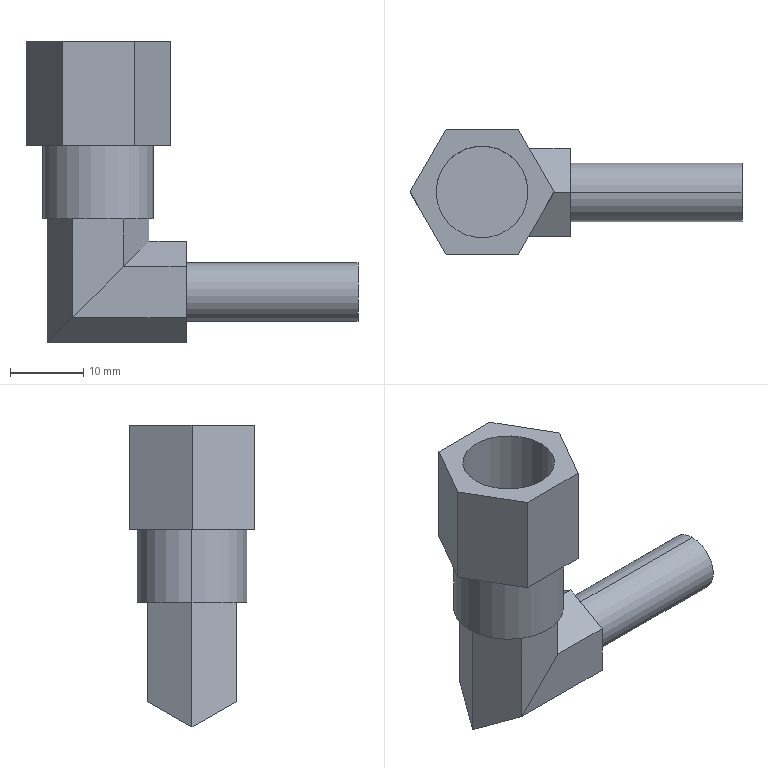Part | STEP file | 1 solid | 30 faces | box 45.215 x 17 x 41.128 mm | volume 7498 mm3 | plane 24 | cylinder 6 | commonest cylinder face diameters 8 x2 12.5 x2 15 x2
STEP:
#1=CARTESIAN_POINT('',(35.4,0.,-24.));
#2=VERTEX_POINT('',#1);
#3=CARTESIAN_POINT('',(35.4,0.,-16.));
#4=VERTEX_POINT('',#3);
#5=CARTESIAN_POINT('',(35.4,0.,-20.));
#6=DIRECTION('',(1.,0.,0.));
#7=DIRECTION('',(0.,0.,-1.));
#8=AXIS2_PLACEMENT_3D('',#5,#6,#7);
#9=CIRCLE('',#8,4.);
#10=EDGE_CURVE('',#2,#4,#9,.T.);
#11=ORIENTED_EDGE('',*,*,#10,.F.);
#12=CARTESIAN_POINT('',(12.,0.,-24.));
#13=VERTEX_POINT('',#12);
#14=CARTESIAN_POINT('',(35.4,0.,-24.));
#15=DIRECTION('',(-1.,0.,0.));
#16=VECTOR('',#15,1000.);
#17=LINE('',#14,#16);
#18=EDGE_CURVE('',#2,#13,#17,.T.);
#19=ORIENTED_EDGE('',*,*,#18,.T.);
#20=CARTESIAN_POINT('',(12.,0.,-16.));
#21=VERTEX_POINT('',#20);
#22=CARTESIAN_POINT('',(12.,0.,-20.));
#23=DIRECTION('',(1.,0.,0.));
#24=DIRECTION('',(0.,0.,-1.));
#25=AXIS2_PLACEMENT_3D('',#22,#23,#24);
#26=CIRCLE('',#25,4.);
#27=EDGE_CURVE('',#13,#21,#26,.T.);
#28=ORIENTED_EDGE('',*,*,#27,.T.);
#29=CARTESIAN_POINT('',(35.4,0.,-16.));
#30=DIRECTION('',(-1.,0.,0.));
#31=VECTOR('',#30,1000.);
#32=LINE('',#29,#31);
#33=EDGE_CURVE('',#4,#21,#32,.T.);
#34=ORIENTED_EDGE('',*,*,#33,.F.);
#35=EDGE_LOOP('',(#11,#19,#28,#34));
#36=FACE_OUTER_BOUND('',#35,.T.);
#37=CARTESIAN_POINT('',(35.4,0.,-20.));
#38=DIRECTION('',(-1.,0.,0.));
#39=DIRECTION('',(0.,0.,1.));
#40=AXIS2_PLACEMENT_3D('',#37,#38,#39);
#41=CYLINDRICAL_SURFACE('',#40,4.);
#42=ADVANCED_FACE('',(#36),#41,.T.);
#43=CARTESIAN_POINT('',(-7.5,0.,-10.));
#44=VERTEX_POINT('',#43);
#45=CARTESIAN_POINT('',(7.5,0.,-10.));
#46=VERTEX_POINT('',#45);
#47=CARTESIAN_POINT('',(0.,0.,-10.));
#48=DIRECTION('',(0.,0.,-1.));
#49=DIRECTION('',(-1.,0.,0.));
#50=AXIS2_PLACEMENT_3D('',#47,#48,#49);
#51=CIRCLE('',#50,7.5);
#52=EDGE_CURVE('',#44,#46,#51,.T.);
#53=ORIENTED_EDGE('',*,*,#52,.F.);
#54=CARTESIAN_POINT('',(-7.5,0.,0.));
#55=VERTEX_POINT('',#54);
#56=CARTESIAN_POINT('',(-7.5,0.,-10.));
#57=DIRECTION('',(0.,0.,1.));
#58=VECTOR('',#57,1000.);
#59=LINE('',#56,#58);
#60=EDGE_CURVE('',#44,#55,#59,.T.);
#61=ORIENTED_EDGE('',*,*,#60,.T.);
#62=CARTESIAN_POINT('',(7.5,0.,0.));
#63=VERTEX_POINT('',#62);
#64=CARTESIAN_POINT('',(0.,0.,0.));
#65=DIRECTION('',(0.,0.,-1.));
#66=DIRECTION('',(1.,0.,0.));
#67=AXIS2_PLACEMENT_3D('',#64,#65,#66);
#68=CIRCLE('',#67,7.5);
#69=EDGE_CURVE('',#55,#63,#68,.T.);
#70=ORIENTED_EDGE('',*,*,#69,.T.);
#71=CARTESIAN_POINT('',(7.5,0.,-10.));
#72=DIRECTION('',(0.,0.,1.));
#73=VECTOR('',#72,1000.);
#74=LINE('',#71,#73);
#75=EDGE_CURVE('',#46,#63,#74,.T.);
#76=ORIENTED_EDGE('',*,*,#75,.F.);
#77=EDGE_LOOP('',(#53,#61,#70,#76));
#78=FACE_OUTER_BOUND('',#77,.T.);
#79=CARTESIAN_POINT('',(0.,0.,-10.));
#80=DIRECTION('',(0.,0.,1.));
#81=DIRECTION('',(1.,0.,0.));
#82=AXIS2_PLACEMENT_3D('',#79,#80,#81);
#83=CYLINDRICAL_SURFACE('',#82,7.5);
#84=ADVANCED_FACE('',(#78),#83,.T.);
#85=CARTESIAN_POINT('',(-6.25,0.,0.));
#86=VERTEX_POINT('',#85);
#87=CARTESIAN_POINT('',(6.25,0.,0.));
#88=VERTEX_POINT('',#87);
#89=CARTESIAN_POINT('',(0.,0.,0.));
#90=DIRECTION('',(0.,0.,1.));
#91=DIRECTION('',(1.,0.,0.));
#92=AXIS2_PLACEMENT_3D('',#89,#90,#91);
#93=CIRCLE('',#92,6.25);
#94=EDGE_CURVE('',#86,#88,#93,.T.);
#95=ORIENTED_EDGE('',*,*,#94,.F.);
#96=CARTESIAN_POINT('',(-6.25,0.,14.2));
#97=VERTEX_POINT('',#96);
#98=CARTESIAN_POINT('',(-6.25,0.,14.2));
#99=DIRECTION('',(0.,0.,1.));
#100=VECTOR('',#99,1000.);
#101=LINE('',#98,#100);
#102=EDGE_CURVE('',#86,#97,#101,.T.);
#103=ORIENTED_EDGE('',*,*,#102,.T.);
#104=CARTESIAN_POINT('',(6.25,0.,14.2));
#105=VERTEX_POINT('',#104);
#106=CARTESIAN_POINT('',(0.,0.,14.2));
#107=DIRECTION('',(0.,0.,1.));
#108=DIRECTION('',(1.,0.,0.));
#109=AXIS2_PLACEMENT_3D('',#106,#107,#108);
#110=CIRCLE('',#109,6.25);
#111=EDGE_CURVE('',#97,#105,#110,.T.);
#112=ORIENTED_EDGE('',*,*,#111,.T.);
#113=CARTESIAN_POINT('',(6.25,0.,14.2));
#114=DIRECTION('',(0.,0.,1.));
#115=VECTOR('',#114,1000.);
#116=LINE('',#113,#115);
#117=EDGE_CURVE('',#88,#105,#116,.T.);
#118=ORIENTED_EDGE('',*,*,#117,.F.);
#119=EDGE_LOOP('',(#95,#103,#112,#118));
#120=FACE_OUTER_BOUND('',#119,.T.);
#121=CARTESIAN_POINT('',(0.,0.,14.2));
#122=DIRECTION('',(0.,0.,1.));
#123=DIRECTION('',(1.,0.,0.));
#124=AXIS2_PLACEMENT_3D('',#121,#122,#123);
#125=CYLINDRICAL_SURFACE('',#124,6.25);
#126=ADVANCED_FACE('',(#120),#125,.F.);
#127=CARTESIAN_POINT('',(4.907,-8.5,0.));
#128=VERTEX_POINT('',#127);
#129=CARTESIAN_POINT('',(9.815,0.,0.));
#130=VERTEX_POINT('',#129);
#131=CARTESIAN_POINT('',(4.907,-8.5,0.));
#132=DIRECTION('',(0.5,0.866,0.));
#133=VECTOR('',#132,1000.);
#134=LINE('',#131,#133);
#135=EDGE_CURVE('',#128,#130,#134,.T.);
#136=ORIENTED_EDGE('',*,*,#135,.T.);
#137=CARTESIAN_POINT('',(9.815,0.,14.2));
#138=VERTEX_POINT('',#137);
#139=CARTESIAN_POINT('',(9.815,0.,14.2));
#140=DIRECTION('',(0.,0.,-1.));
#141=VECTOR('',#140,1000.);
#142=LINE('',#139,#141);
#143=EDGE_CURVE('',#138,#130,#142,.T.);
#144=ORIENTED_EDGE('',*,*,#143,.F.);
#145=CARTESIAN_POINT('',(4.907,-8.5,14.2));
#146=VERTEX_POINT('',#145);
#147=CARTESIAN_POINT('',(4.907,-8.5,14.2));
#148=DIRECTION('',(0.5,0.866,0.));
#149=VECTOR('',#148,1000.);
#150=LINE('',#147,#149);
#151=EDGE_CURVE('',#146,#138,#150,.T.);
#152=ORIENTED_EDGE('',*,*,#151,.F.);
#153=CARTESIAN_POINT('',(4.907,-8.5,14.2));
#154=DIRECTION('',(0.,0.,-1.));
#155=VECTOR('',#154,1000.);
#156=LINE('',#153,#155);
#157=EDGE_CURVE('',#146,#128,#156,.T.);
#158=ORIENTED_EDGE('',*,*,#157,.T.);
#159=EDGE_LOOP('',(#136,#144,#152,#158));
#160=FACE_OUTER_BOUND('',#159,.T.);
#161=CARTESIAN_POINT('',(4.907,-8.5,14.2));
#162=DIRECTION('',(-0.866,0.5,0.));
#163=DIRECTION('',(-0.5,-0.866,0.));
#164=AXIS2_PLACEMENT_3D('',#161,#162,#163);
#165=PLANE('',#164);
#166=ADVANCED_FACE('',(#160),#165,.F.);
#167=CARTESIAN_POINT('',(4.907,8.5,0.));
#168=VERTEX_POINT('',#167);
#169=CARTESIAN_POINT('',(9.815,0.,0.));
#170=DIRECTION('',(-0.5,0.866,0.));
#171=VECTOR('',#170,1000.);
#172=LINE('',#169,#171);
#173=EDGE_CURVE('',#130,#168,#172,.T.);
#174=ORIENTED_EDGE('',*,*,#173,.T.);
#175=CARTESIAN_POINT('',(4.907,8.5,14.2));
#176=VERTEX_POINT('',#175);
#177=CARTESIAN_POINT('',(4.907,8.5,14.2));
#178=DIRECTION('',(0.,0.,-1.));
#179=VECTOR('',#178,1000.);
#180=LINE('',#177,#179);
#181=EDGE_CURVE('',#176,#168,#180,.T.);
#182=ORIENTED_EDGE('',*,*,#181,.F.);
#183=CARTESIAN_POINT('',(9.815,0.,14.2));
#184=DIRECTION('',(-0.5,0.866,0.));
#185=VECTOR('',#184,1000.);
#186=LINE('',#183,#185);
#187=EDGE_CURVE('',#138,#176,#186,.T.);
#188=ORIENTED_EDGE('',*,*,#187,.F.);
#189=ORIENTED_EDGE('',*,*,#143,.T.);
#190=EDGE_LOOP('',(#174,#182,#188,#189));
#191=FACE_OUTER_BOUND('',#190,.T.);
#192=CARTESIAN_POINT('',(9.815,0.,14.2));
#193=DIRECTION('',(-0.866,-0.5,0.));
#194=DIRECTION('',(0.5,-0.866,0.));
#195=AXIS2_PLACEMENT_3D('',#192,#193,#194);
#196=PLANE('',#195);
#197=ADVANCED_FACE('',(#191),#196,.F.);
#198=CARTESIAN_POINT('',(-4.907,8.5,0.));
#199=VERTEX_POINT('',#198);
#200=CARTESIAN_POINT('',(4.907,8.5,0.));
#201=DIRECTION('',(-1.,0.,0.));
#202=VECTOR('',#201,1000.);
#203=LINE('',#200,#202);
#204=EDGE_CURVE('',#168,#199,#203,.T.);
#205=ORIENTED_EDGE('',*,*,#204,.T.);
#206=CARTESIAN_POINT('',(-4.907,8.5,14.2));
#207=VERTEX_POINT('',#206);
#208=CARTESIAN_POINT('',(-4.907,8.5,14.2));
#209=DIRECTION('',(0.,0.,-1.));
#210=VECTOR('',#209,1000.);
#211=LINE('',#208,#210);
#212=EDGE_CURVE('',#207,#199,#211,.T.);
#213=ORIENTED_EDGE('',*,*,#212,.F.);
#214=CARTESIAN_POINT('',(4.907,8.5,14.2));
#215=DIRECTION('',(-1.,0.,0.));
#216=VECTOR('',#215,1000.);
#217=LINE('',#214,#216);
#218=EDGE_CURVE('',#176,#207,#217,.T.);
#219=ORIENTED_EDGE('',*,*,#218,.F.);
#220=ORIENTED_EDGE('',*,*,#181,.T.);
#221=EDGE_LOOP('',(#205,#213,#219,#220));
#222=FACE_OUTER_BOUND('',#221,.T.);
#223=CARTESIAN_POINT('',(4.907,8.5,14.2));
#224=DIRECTION('',(0.,-1.,0.));
#225=DIRECTION('',(1.,0.,0.));
#226=AXIS2_PLACEMENT_3D('',#223,#224,#225);
#227=PLANE('',#226);
#228=ADVANCED_FACE('',(#222),#227,.F.);
#229=CARTESIAN_POINT('',(-9.815,0.,0.));
#230=VERTEX_POINT('',#229);
#231=CARTESIAN_POINT('',(-4.907,8.5,0.));
#232=DIRECTION('',(-0.5,-0.866,0.));
#233=VECTOR('',#232,1000.);
#234=LINE('',#231,#233);
#235=EDGE_CURVE('',#199,#230,#234,.T.);
#236=ORIENTED_EDGE('',*,*,#235,.T.);
#237=CARTESIAN_POINT('',(-9.815,0.,14.2));
#238=VERTEX_POINT('',#237);
#239=CARTESIAN_POINT('',(-9.815,0.,14.2));
#240=DIRECTION('',(0.,0.,-1.));
#241=VECTOR('',#240,1000.);
#242=LINE('',#239,#241);
#243=EDGE_CURVE('',#238,#230,#242,.T.);
#244=ORIENTED_EDGE('',*,*,#243,.F.);
#245=CARTESIAN_POINT('',(-4.907,8.5,14.2));
#246=DIRECTION('',(-0.5,-0.866,0.));
#247=VECTOR('',#246,1000.);
#248=LINE('',#245,#247);
#249=EDGE_CURVE('',#207,#238,#248,.T.);
#250=ORIENTED_EDGE('',*,*,#249,.F.);
#251=ORIENTED_EDGE('',*,*,#212,.T.);
#252=EDGE_LOOP('',(#236,#244,#250,#251));
#253=FACE_OUTER_BOUND('',#252,.T.);
#254=CARTESIAN_POINT('',(-4.907,8.5,14.2));
#255=DIRECTION('',(0.866,-0.5,0.));
#256=DIRECTION('',(0.5,0.866,0.));
#257=AXIS2_PLACEMENT_3D('',#254,#255,#256);
#258=PLANE('',#257);
#259=ADVANCED_FACE('',(#253),#258,.F.);
#260=CARTESIAN_POINT('',(-4.907,-8.5,0.));
#261=VERTEX_POINT('',#260);
#262=CARTESIAN_POINT('',(-9.815,0.,0.));
#263=DIRECTION('',(0.5,-0.866,0.));
#264=VECTOR('',#263,1000.);
#265=LINE('',#262,#264);
#266=EDGE_CURVE('',#230,#261,#265,.T.);
#267=ORIENTED_EDGE('',*,*,#266,.T.);
#268=CARTESIAN_POINT('',(-4.907,-8.5,14.2));
#269=VERTEX_POINT('',#268);
#270=CARTESIAN_POINT('',(-4.907,-8.5,14.2));
#271=DIRECTION('',(0.,0.,-1.));
#272=VECTOR('',#271,1000.);
#273=LINE('',#270,#272);
#274=EDGE_CURVE('',#269,#261,#273,.T.);
#275=ORIENTED_EDGE('',*,*,#274,.F.);
#276=CARTESIAN_POINT('',(-9.815,0.,14.2));
#277=DIRECTION('',(0.5,-0.866,0.));
#278=VECTOR('',#277,1000.);
#279=LINE('',#276,#278);
#280=EDGE_CURVE('',#238,#269,#279,.T.);
#281=ORIENTED_EDGE('',*,*,#280,.F.);
#282=ORIENTED_EDGE('',*,*,#243,.T.);
#283=EDGE_LOOP('',(#267,#275,#281,#282));
#284=FACE_OUTER_BOUND('',#283,.T.);
#285=CARTESIAN_POINT('',(-9.815,0.,14.2));
#286=DIRECTION('',(0.866,0.5,0.));
#287=DIRECTION('',(-0.5,0.866,0.));
#288=AXIS2_PLACEMENT_3D('',#285,#286,#287);
#289=PLANE('',#288);
#290=ADVANCED_FACE('',(#284),#289,.F.);
#291=CARTESIAN_POINT('',(-4.907,-8.5,0.));
#292=DIRECTION('',(1.,0.,0.));
#293=VECTOR('',#292,1000.);
#294=LINE('',#291,#293);
#295=EDGE_CURVE('',#261,#128,#294,.T.);
#296=ORIENTED_EDGE('',*,*,#295,.T.);
#297=ORIENTED_EDGE('',*,*,#157,.F.);
#298=CARTESIAN_POINT('',(-4.907,-8.5,14.2));
#299=DIRECTION('',(1.,0.,0.));
#300=VECTOR('',#299,1000.);
#301=LINE('',#298,#300);
#302=EDGE_CURVE('',#269,#146,#301,.T.);
#303=ORIENTED_EDGE('',*,*,#302,.F.);
#304=ORIENTED_EDGE('',*,*,#274,.T.);
#305=EDGE_LOOP('',(#296,#297,#303,#304));
#306=FACE_OUTER_BOUND('',#305,.T.);
#307=CARTESIAN_POINT('',(-4.907,-8.5,14.2));
#308=DIRECTION('',(0.,1.,0.));
#309=DIRECTION('',(-1.,0.,0.));
#310=AXIS2_PLACEMENT_3D('',#307,#308,#309);
#311=PLANE('',#310);
#312=ADVANCED_FACE('',(#306),#311,.F.);
#313=CARTESIAN_POINT('',(0.,0.,14.2));
#314=DIRECTION('',(0.,0.,1.));
#315=DIRECTION('',(1.,0.,0.));
#316=AXIS2_PLACEMENT_3D('',#313,#314,#315);
#317=CIRCLE('',#316,6.25);
#318=EDGE_CURVE('',#105,#97,#317,.T.);
#319=ORIENTED_EDGE('',*,*,#318,.F.);
#320=ORIENTED_EDGE('',*,*,#111,.F.);
#321=EDGE_LOOP('',(#319,#320));
#322=FACE_BOUND('',#321,.T.);
#323=ORIENTED_EDGE('',*,*,#151,.T.);
#324=ORIENTED_EDGE('',*,*,#187,.T.);
#325=ORIENTED_EDGE('',*,*,#218,.T.);
#326=ORIENTED_EDGE('',*,*,#249,.T.);
#327=ORIENTED_EDGE('',*,*,#280,.T.);
#328=ORIENTED_EDGE('',*,*,#302,.T.);
#329=EDGE_LOOP('',(#323,#324,#325,#326,#327,#328));
#330=FACE_OUTER_BOUND('',#329,.T.);
#331=CARTESIAN_POINT('',(0.,0.,14.2));
#332=DIRECTION('',(0.,0.,1.));
#333=DIRECTION('',(1.,0.,0.));
#334=AXIS2_PLACEMENT_3D('',#331,#332,#333);
#335=PLANE('',#334);
#336=ADVANCED_FACE('',(#322,#330),#335,.T.);
#337=CARTESIAN_POINT('',(0.,0.,0.));
#338=DIRECTION('',(0.,0.,-1.));
#339=DIRECTION('',(1.,0.,0.));
#340=AXIS2_PLACEMENT_3D('',#337,#338,#339);
#341=CIRCLE('',#340,7.5);
#342=EDGE_CURVE('',#63,#55,#341,.T.);
#343=ORIENTED_EDGE('',*,*,#342,.F.);
#344=ORIENTED_EDGE('',*,*,#69,.F.);
#345=EDGE_LOOP('',(#343,#344));
#346=FACE_BOUND('',#345,.T.);
#347=ORIENTED_EDGE('',*,*,#135,.F.);
#348=ORIENTED_EDGE('',*,*,#295,.F.);
#349=ORIENTED_EDGE('',*,*,#266,.F.);
#350=ORIENTED_EDGE('',*,*,#235,.F.);
#351=ORIENTED_EDGE('',*,*,#204,.F.);
#352=ORIENTED_EDGE('',*,*,#173,.F.);
#353=EDGE_LOOP('',(#347,#348,#349,#350,#351,#352));
#354=FACE_OUTER_BOUND('',#353,.T.);
#355=CARTESIAN_POINT('',(0.,0.,0.));
#356=DIRECTION('',(0.,0.,1.));
#357=DIRECTION('',(1.,0.,0.));
#358=AXIS2_PLACEMENT_3D('',#355,#356,#357);
#359=PLANE('',#358);
#360=ADVANCED_FACE('',(#346,#354),#359,.F.);
#361=ORIENTED_EDGE('',*,*,#102,.F.);
#362=CARTESIAN_POINT('',(0.,0.,0.));
#363=DIRECTION('',(0.,0.,1.));
#364=DIRECTION('',(1.,0.,0.));
#365=AXIS2_PLACEMENT_3D('',#362,#363,#364);
#366=CIRCLE('',#365,6.25);
#367=EDGE_CURVE('',#88,#86,#366,.T.);
#368=ORIENTED_EDGE('',*,*,#367,.F.);
#369=ORIENTED_EDGE('',*,*,#117,.T.);
#370=ORIENTED_EDGE('',*,*,#318,.T.);
#371=EDGE_LOOP('',(#361,#368,#369,#370));
#372=FACE_OUTER_BOUND('',#371,.T.);
#373=CARTESIAN_POINT('',(0.,0.,14.2));
#374=DIRECTION('',(0.,0.,1.));
#375=DIRECTION('',(1.,0.,0.));
#376=AXIS2_PLACEMENT_3D('',#373,#374,#375);
#377=CYLINDRICAL_SURFACE('',#376,6.25);
#378=ADVANCED_FACE('',(#372),#377,.F.);
#379=ORIENTED_EDGE('',*,*,#367,.T.);
#380=ORIENTED_EDGE('',*,*,#94,.T.);
#381=EDGE_LOOP('',(#379,#380));
#382=FACE_OUTER_BOUND('',#381,.T.);
#383=CARTESIAN_POINT('',(0.,0.,0.));
#384=DIRECTION('',(0.,0.,-1.));
#385=DIRECTION('',(-1.,0.,0.));
#386=AXIS2_PLACEMENT_3D('',#383,#384,#385);
#387=PLANE('',#386);
#388=ADVANCED_FACE('',(#382),#387,.F.);
#389=ORIENTED_EDGE('',*,*,#60,.F.);
#390=CARTESIAN_POINT('',(0.,0.,-10.));
#391=DIRECTION('',(0.,0.,-1.));
#392=DIRECTION('',(-1.,0.,0.));
#393=AXIS2_PLACEMENT_3D('',#390,#391,#392);
#394=CIRCLE('',#393,7.5);
#395=EDGE_CURVE('',#46,#44,#394,.T.);
#396=ORIENTED_EDGE('',*,*,#395,.F.);
#397=ORIENTED_EDGE('',*,*,#75,.T.);
#398=ORIENTED_EDGE('',*,*,#342,.T.);
#399=EDGE_LOOP('',(#389,#396,#397,#398));
#400=FACE_OUTER_BOUND('',#399,.T.);
#401=CARTESIAN_POINT('',(0.,0.,-10.));
#402=DIRECTION('',(0.,0.,1.));
#403=DIRECTION('',(1.,0.,0.));
#404=AXIS2_PLACEMENT_3D('',#401,#402,#403);
#405=CYLINDRICAL_SURFACE('',#404,7.5);
#406=ADVANCED_FACE('',(#400),#405,.T.);
#407=CARTESIAN_POINT('',(-3.464,-6.,-10.));
#408=VERTEX_POINT('',#407);
#409=CARTESIAN_POINT('',(-6.928,0.,-10.));
#410=VERTEX_POINT('',#409);
#411=CARTESIAN_POINT('',(-3.464,-6.,-10.));
#412=DIRECTION('',(-0.5,0.866,0.));
#413=VECTOR('',#412,1000.);
#414=LINE('',#411,#413);
#415=EDGE_CURVE('',#408,#410,#414,.T.);
#416=ORIENTED_EDGE('',*,*,#415,.F.);
#417=CARTESIAN_POINT('',(3.464,-6.,-10.));
#418=VERTEX_POINT('',#417);
#419=CARTESIAN_POINT('',(3.464,-6.,-10.));
#420=DIRECTION('',(-1.,0.,0.));
#421=VECTOR('',#420,1000.);
#422=LINE('',#419,#421);
#423=EDGE_CURVE('',#418,#408,#422,.T.);
#424=ORIENTED_EDGE('',*,*,#423,.F.);
#425=CARTESIAN_POINT('',(6.928,0.,-10.));
#426=VERTEX_POINT('',#425);
#427=CARTESIAN_POINT('',(6.928,0.,-10.));
#428=DIRECTION('',(-0.5,-0.866,0.));
#429=VECTOR('',#428,1000.);
#430=LINE('',#427,#429);
#431=EDGE_CURVE('',#426,#418,#430,.T.);
#432=ORIENTED_EDGE('',*,*,#431,.F.);
#433=CARTESIAN_POINT('',(3.464,6.,-10.));
#434=VERTEX_POINT('',#433);
#435=CARTESIAN_POINT('',(3.464,6.,-10.));
#436=DIRECTION('',(0.5,-0.866,0.));
#437=VECTOR('',#436,1000.);
#438=LINE('',#435,#437);
#439=EDGE_CURVE('',#434,#426,#438,.T.);
#440=ORIENTED_EDGE('',*,*,#439,.F.);
#441=CARTESIAN_POINT('',(-3.464,6.,-10.));
#442=VERTEX_POINT('',#441);
#443=CARTESIAN_POINT('',(-3.464,6.,-10.));
#444=DIRECTION('',(1.,0.,0.));
#445=VECTOR('',#444,1000.);
#446=LINE('',#443,#445);
#447=EDGE_CURVE('',#442,#434,#446,.T.);
#448=ORIENTED_EDGE('',*,*,#447,.F.);
#449=CARTESIAN_POINT('',(-6.928,0.,-10.));
#450=DIRECTION('',(0.5,0.866,0.));
#451=VECTOR('',#450,1000.);
#452=LINE('',#449,#451);
#453=EDGE_CURVE('',#410,#442,#452,.T.);
#454=ORIENTED_EDGE('',*,*,#453,.F.);
#455=EDGE_LOOP('',(#416,#424,#432,#440,#448,#454));
#456=FACE_BOUND('',#455,.T.);
#457=ORIENTED_EDGE('',*,*,#395,.T.);
#458=ORIENTED_EDGE('',*,*,#52,.T.);
#459=EDGE_LOOP('',(#457,#458));
#460=FACE_OUTER_BOUND('',#459,.T.);
#461=CARTESIAN_POINT('',(0.,0.,-10.));
#462=DIRECTION('',(0.,0.,-1.));
#463=DIRECTION('',(-1.,0.,0.));
#464=AXIS2_PLACEMENT_3D('',#461,#462,#463);
#465=PLANE('',#464);
#466=ADVANCED_FACE('',(#456,#460),#465,.T.);
#467=CARTESIAN_POINT('',(-6.928,0.,-26.928));
#468=VERTEX_POINT('',#467);
#469=CARTESIAN_POINT('',(-6.928,0.,-10.));
#470=DIRECTION('',(0.,0.,-1.));
#471=VECTOR('',#470,1000.);
#472=LINE('',#469,#471);
#473=EDGE_CURVE('',#410,#468,#472,.T.);
#474=ORIENTED_EDGE('',*,*,#473,.T.);
#475=CARTESIAN_POINT('',(-3.464,-6.,-23.464));
#476=VERTEX_POINT('',#475);
#477=CARTESIAN_POINT('',(-0.7713,-10.664,-20.771));
#478=DIRECTION('',(0.4472,-0.7746,0.4472));
#479=VECTOR('',#478,1000.);
#480=LINE('',#477,#479);
#481=EDGE_CURVE('',#468,#476,#480,.T.);
#482=ORIENTED_EDGE('',*,*,#481,.T.);
#483=CARTESIAN_POINT('',(-3.464,-6.,-10.));
#484=DIRECTION('',(0.,0.,-1.));
#485=VECTOR('',#484,1000.);
#486=LINE('',#483,#485);
#487=EDGE_CURVE('',#408,#476,#486,.T.);
#488=ORIENTED_EDGE('',*,*,#487,.F.);
#489=ORIENTED_EDGE('',*,*,#415,.T.);
#490=EDGE_LOOP('',(#474,#482,#488,#489));
#491=FACE_OUTER_BOUND('',#490,.T.);
#492=CARTESIAN_POINT('',(-3.464,-6.,-10.));
#493=DIRECTION('',(-0.866,-0.5,0.));
#494=DIRECTION('',(0.5,-0.866,0.));
#495=AXIS2_PLACEMENT_3D('',#492,#493,#494);
#496=PLANE('',#495);
#497=ADVANCED_FACE('',(#491),#496,.T.);
#498=CARTESIAN_POINT('',(-3.464,6.,-23.464));
#499=VERTEX_POINT('',#498);
#500=CARTESIAN_POINT('',(-3.464,6.,-10.));
#501=DIRECTION('',(0.,0.,-1.));
#502=VECTOR('',#501,1000.);
#503=LINE('',#500,#502);
#504=EDGE_CURVE('',#442,#499,#503,.T.);
#505=ORIENTED_EDGE('',*,*,#504,.T.);
#506=CARTESIAN_POINT('',(-3.543,5.864,-23.543));
#507=DIRECTION('',(-0.4472,-0.7746,-0.4472));
#508=VECTOR('',#507,1000.);
#509=LINE('',#506,#508);
#510=EDGE_CURVE('',#499,#468,#509,.T.);
#511=ORIENTED_EDGE('',*,*,#510,.T.);
#512=ORIENTED_EDGE('',*,*,#473,.F.);
#513=ORIENTED_EDGE('',*,*,#453,.T.);
#514=EDGE_LOOP('',(#505,#511,#512,#513));
#515=FACE_OUTER_BOUND('',#514,.T.);
#516=CARTESIAN_POINT('',(-6.928,0.,-10.));
#517=DIRECTION('',(-0.866,0.5,0.));
#518=DIRECTION('',(-0.5,-0.866,0.));
#519=AXIS2_PLACEMENT_3D('',#516,#517,#518);
#520=PLANE('',#519);
#521=ADVANCED_FACE('',(#515),#520,.T.);
#522=CARTESIAN_POINT('',(3.464,6.,-16.536));
#523=VERTEX_POINT('',#522);
#524=CARTESIAN_POINT('',(3.464,6.,-10.));
#525=DIRECTION('',(0.,0.,-1.));
#526=VECTOR('',#525,1000.);
#527=LINE('',#524,#526);
#528=EDGE_CURVE('',#434,#523,#527,.T.);
#529=ORIENTED_EDGE('',*,*,#528,.T.);
#530=CARTESIAN_POINT('',(3.268,6.,-16.732));
#531=DIRECTION('',(-0.7071,0.,-0.7071));
#532=VECTOR('',#531,1000.);
#533=LINE('',#530,#532);
#534=EDGE_CURVE('',#523,#499,#533,.T.);
#535=ORIENTED_EDGE('',*,*,#534,.T.);
#536=ORIENTED_EDGE('',*,*,#504,.F.);
#537=ORIENTED_EDGE('',*,*,#447,.T.);
#538=EDGE_LOOP('',(#529,#535,#536,#537));
#539=FACE_OUTER_BOUND('',#538,.T.);
#540=CARTESIAN_POINT('',(-3.464,6.,-10.));
#541=DIRECTION('',(0.,1.,0.));
#542=DIRECTION('',(-1.,0.,0.));
#543=AXIS2_PLACEMENT_3D('',#540,#541,#542);
#544=PLANE('',#543);
#545=ADVANCED_FACE('',(#539),#544,.T.);
#546=CARTESIAN_POINT('',(6.928,0.,-13.072));
#547=VERTEX_POINT('',#546);
#548=CARTESIAN_POINT('',(6.928,0.,-10.));
#549=DIRECTION('',(0.,0.,-1.));
#550=VECTOR('',#549,1000.);
#551=LINE('',#548,#550);
#552=EDGE_CURVE('',#426,#547,#551,.T.);
#553=ORIENTED_EDGE('',*,*,#552,.T.);
#554=CARTESIAN_POINT('',(4.771,3.736,-15.229));
#555=DIRECTION('',(-0.4472,0.7746,-0.4472));
#556=VECTOR('',#555,1000.);
#557=LINE('',#554,#556);
#558=EDGE_CURVE('',#547,#523,#557,.T.);
#559=ORIENTED_EDGE('',*,*,#558,.T.);
#560=ORIENTED_EDGE('',*,*,#528,.F.);
#561=ORIENTED_EDGE('',*,*,#439,.T.);
#562=EDGE_LOOP('',(#553,#559,#560,#561));
#563=FACE_OUTER_BOUND('',#562,.T.);
#564=CARTESIAN_POINT('',(3.464,6.,-10.));
#565=DIRECTION('',(0.866,0.5,0.));
#566=DIRECTION('',(-0.5,0.866,0.));
#567=AXIS2_PLACEMENT_3D('',#564,#565,#566);
#568=PLANE('',#567);
#569=ADVANCED_FACE('',(#563),#568,.T.);
#570=CARTESIAN_POINT('',(3.464,-6.,-16.536));
#571=VERTEX_POINT('',#570);
#572=CARTESIAN_POINT('',(3.464,-6.,-10.));
#573=DIRECTION('',(0.,0.,-1.));
#574=VECTOR('',#573,1000.);
#575=LINE('',#572,#574);
#576=EDGE_CURVE('',#418,#571,#575,.T.);
#577=ORIENTED_EDGE('',*,*,#576,.T.);
#578=CARTESIAN_POINT('',(7.543,1.064,-12.457));
#579=DIRECTION('',(0.4472,0.7746,0.4472));
#580=VECTOR('',#579,1000.);
#581=LINE('',#578,#580);
#582=EDGE_CURVE('',#571,#547,#581,.T.);
#583=ORIENTED_EDGE('',*,*,#582,.T.);
#584=ORIENTED_EDGE('',*,*,#552,.F.);
#585=ORIENTED_EDGE('',*,*,#431,.T.);
#586=EDGE_LOOP('',(#577,#583,#584,#585));
#587=FACE_OUTER_BOUND('',#586,.T.);
#588=CARTESIAN_POINT('',(6.928,0.,-10.));
#589=DIRECTION('',(0.866,-0.5,0.));
#590=DIRECTION('',(0.5,0.866,0.));
#591=AXIS2_PLACEMENT_3D('',#588,#589,#590);
#592=PLANE('',#591);
#593=ADVANCED_FACE('',(#587),#592,.T.);
#594=ORIENTED_EDGE('',*,*,#487,.T.);
#595=CARTESIAN_POINT('',(6.732,-6.,-13.268));
#596=DIRECTION('',(0.7071,0.,0.7071));
#597=VECTOR('',#596,1000.);
#598=LINE('',#595,#597);
#599=EDGE_CURVE('',#476,#571,#598,.T.);
#600=ORIENTED_EDGE('',*,*,#599,.T.);
#601=ORIENTED_EDGE('',*,*,#576,.F.);
#602=ORIENTED_EDGE('',*,*,#423,.T.);
#603=EDGE_LOOP('',(#594,#600,#601,#602));
#604=FACE_OUTER_BOUND('',#603,.T.);
#605=CARTESIAN_POINT('',(3.464,-6.,-10.));
#606=DIRECTION('',(0.,-1.,0.));
#607=DIRECTION('',(1.,0.,0.));
#608=AXIS2_PLACEMENT_3D('',#605,#606,#607);
#609=PLANE('',#608);
#610=ADVANCED_FACE('',(#604),#609,.T.);
#611=ORIENTED_EDGE('',*,*,#599,.F.);
#612=CARTESIAN_POINT('',(12.,-6.,-23.464));
#613=VERTEX_POINT('',#612);
#614=CARTESIAN_POINT('',(-7.721,-6.,-23.464));
#615=DIRECTION('',(1.,0.,0.));
#616=VECTOR('',#615,1000.);
#617=LINE('',#614,#616);
#618=EDGE_CURVE('',#476,#613,#617,.T.);
#619=ORIENTED_EDGE('',*,*,#618,.T.);
#620=CARTESIAN_POINT('',(12.,-6.,-16.536));
#621=VERTEX_POINT('',#620);
#622=CARTESIAN_POINT('',(12.,-6.,-16.536));
#623=DIRECTION('',(0.,0.,-1.));
#624=VECTOR('',#623,1000.);
#625=LINE('',#622,#624);
#626=EDGE_CURVE('',#621,#613,#625,.T.);
#627=ORIENTED_EDGE('',*,*,#626,.F.);
#628=CARTESIAN_POINT('',(-7.721,-6.,-16.536));
#629=DIRECTION('',(1.,0.,0.));
#630=VECTOR('',#629,1000.);
#631=LINE('',#628,#630);
#632=EDGE_CURVE('',#571,#621,#631,.T.);
#633=ORIENTED_EDGE('',*,*,#632,.F.);
#634=EDGE_LOOP('',(#611,#619,#627,#633));
#635=FACE_OUTER_BOUND('',#634,.T.);
#636=CARTESIAN_POINT('',(-7.721,-6.,-16.536));
#637=DIRECTION('',(0.,-1.,0.));
#638=DIRECTION('',(0.,0.,-1.));
#639=AXIS2_PLACEMENT_3D('',#636,#637,#638);
#640=PLANE('',#639);
#641=ADVANCED_FACE('',(#635),#640,.T.);
#642=ORIENTED_EDGE('',*,*,#582,.F.);
#643=ORIENTED_EDGE('',*,*,#632,.T.);
#644=CARTESIAN_POINT('',(12.,0.,-13.072));
#645=VERTEX_POINT('',#644);
#646=CARTESIAN_POINT('',(12.,0.,-13.072));
#647=DIRECTION('',(0.,-0.866,-0.5));
#648=VECTOR('',#647,1000.);
#649=LINE('',#646,#648);
#650=EDGE_CURVE('',#645,#621,#649,.T.);
#651=ORIENTED_EDGE('',*,*,#650,.F.);
#652=CARTESIAN_POINT('',(-7.721,0.,-13.072));
#653=DIRECTION('',(1.,0.,0.));
#654=VECTOR('',#653,1000.);
#655=LINE('',#652,#654);
#656=EDGE_CURVE('',#547,#645,#655,.T.);
#657=ORIENTED_EDGE('',*,*,#656,.F.);
#658=EDGE_LOOP('',(#642,#643,#651,#657));
#659=FACE_OUTER_BOUND('',#658,.T.);
#660=CARTESIAN_POINT('',(-7.721,0.,-13.072));
#661=DIRECTION('',(0.,-0.5,0.866));
#662=DIRECTION('',(0.,-0.866,-0.5));
#663=AXIS2_PLACEMENT_3D('',#660,#661,#662);
#664=PLANE('',#663);
#665=ADVANCED_FACE('',(#659),#664,.T.);
#666=ORIENTED_EDGE('',*,*,#558,.F.);
#667=ORIENTED_EDGE('',*,*,#656,.T.);
#668=CARTESIAN_POINT('',(12.,6.,-16.536));
#669=VERTEX_POINT('',#668);
#670=CARTESIAN_POINT('',(12.,6.,-16.536));
#671=DIRECTION('',(0.,-0.866,0.5));
#672=VECTOR('',#671,1000.);
#673=LINE('',#670,#672);
#674=EDGE_CURVE('',#669,#645,#673,.T.);
#675=ORIENTED_EDGE('',*,*,#674,.F.);
#676=CARTESIAN_POINT('',(-7.721,6.,-16.536));
#677=DIRECTION('',(1.,0.,0.));
#678=VECTOR('',#677,1000.);
#679=LINE('',#676,#678);
#680=EDGE_CURVE('',#523,#669,#679,.T.);
#681=ORIENTED_EDGE('',*,*,#680,.F.);
#682=EDGE_LOOP('',(#666,#667,#675,#681));
#683=FACE_OUTER_BOUND('',#682,.T.);
#684=CARTESIAN_POINT('',(-7.721,6.,-16.536));
#685=DIRECTION('',(0.,0.5,0.866));
#686=DIRECTION('',(0.,-0.866,0.5));
#687=AXIS2_PLACEMENT_3D('',#684,#685,#686);
#688=PLANE('',#687);
#689=ADVANCED_FACE('',(#683),#688,.T.);
#690=ORIENTED_EDGE('',*,*,#534,.F.);
#691=ORIENTED_EDGE('',*,*,#680,.T.);
#692=CARTESIAN_POINT('',(12.,6.,-23.464));
#693=VERTEX_POINT('',#692);
#694=CARTESIAN_POINT('',(12.,6.,-23.464));
#695=DIRECTION('',(0.,0.,1.));
#696=VECTOR('',#695,1000.);
#697=LINE('',#694,#696);
#698=EDGE_CURVE('',#693,#669,#697,.T.);
#699=ORIENTED_EDGE('',*,*,#698,.F.);
#700=CARTESIAN_POINT('',(-7.721,6.,-23.464));
#701=DIRECTION('',(1.,0.,0.));
#702=VECTOR('',#701,1000.);
#703=LINE('',#700,#702);
#704=EDGE_CURVE('',#499,#693,#703,.T.);
#705=ORIENTED_EDGE('',*,*,#704,.F.);
#706=EDGE_LOOP('',(#690,#691,#699,#705));
#707=FACE_OUTER_BOUND('',#706,.T.);
#708=CARTESIAN_POINT('',(-7.721,6.,-23.464));
#709=DIRECTION('',(0.,1.,0.));
#710=DIRECTION('',(0.,0.,1.));
#711=AXIS2_PLACEMENT_3D('',#708,#709,#710);
#712=PLANE('',#711);
#713=ADVANCED_FACE('',(#707),#712,.T.);
#714=ORIENTED_EDGE('',*,*,#510,.F.);
#715=ORIENTED_EDGE('',*,*,#704,.T.);
#716=CARTESIAN_POINT('',(12.,0.,-26.928));
#717=VERTEX_POINT('',#716);
#718=CARTESIAN_POINT('',(12.,0.,-26.928));
#719=DIRECTION('',(0.,0.866,0.5));
#720=VECTOR('',#719,1000.);
#721=LINE('',#718,#720);
#722=EDGE_CURVE('',#717,#693,#721,.T.);
#723=ORIENTED_EDGE('',*,*,#722,.F.);
#724=CARTESIAN_POINT('',(-7.721,0.,-26.928));
#725=DIRECTION('',(1.,0.,0.));
#726=VECTOR('',#725,1000.);
#727=LINE('',#724,#726);
#728=EDGE_CURVE('',#468,#717,#727,.T.);
#729=ORIENTED_EDGE('',*,*,#728,.F.);
#730=EDGE_LOOP('',(#714,#715,#723,#729));
#731=FACE_OUTER_BOUND('',#730,.T.);
#732=CARTESIAN_POINT('',(-7.721,0.,-26.928));
#733=DIRECTION('',(0.,0.5,-0.866));
#734=DIRECTION('',(0.,0.866,0.5));
#735=AXIS2_PLACEMENT_3D('',#732,#733,#734);
#736=PLANE('',#735);
#737=ADVANCED_FACE('',(#731),#736,.T.);
#738=ORIENTED_EDGE('',*,*,#481,.F.);
#739=ORIENTED_EDGE('',*,*,#728,.T.);
#740=CARTESIAN_POINT('',(12.,-6.,-23.464));
#741=DIRECTION('',(0.,0.866,-0.5));
#742=VECTOR('',#741,1000.);
#743=LINE('',#740,#742);
#744=EDGE_CURVE('',#613,#717,#743,.T.);
#745=ORIENTED_EDGE('',*,*,#744,.F.);
#746=ORIENTED_EDGE('',*,*,#618,.F.);
#747=EDGE_LOOP('',(#738,#739,#745,#746));
#748=FACE_OUTER_BOUND('',#747,.T.);
#749=CARTESIAN_POINT('',(-7.721,-6.,-23.464));
#750=DIRECTION('',(0.,-0.5,-0.866));
#751=DIRECTION('',(0.,0.866,-0.5));
#752=AXIS2_PLACEMENT_3D('',#749,#750,#751);
#753=PLANE('',#752);
#754=ADVANCED_FACE('',(#748),#753,.T.);
#755=CARTESIAN_POINT('',(12.,0.,-20.));
#756=DIRECTION('',(1.,0.,0.));
#757=DIRECTION('',(0.,0.,-1.));
#758=AXIS2_PLACEMENT_3D('',#755,#756,#757);
#759=CIRCLE('',#758,4.);
#760=EDGE_CURVE('',#21,#13,#759,.T.);
#761=ORIENTED_EDGE('',*,*,#760,.F.);
#762=ORIENTED_EDGE('',*,*,#27,.F.);
#763=EDGE_LOOP('',(#761,#762));
#764=FACE_BOUND('',#763,.T.);
#765=ORIENTED_EDGE('',*,*,#744,.T.);
#766=ORIENTED_EDGE('',*,*,#722,.T.);
#767=ORIENTED_EDGE('',*,*,#698,.T.);
#768=ORIENTED_EDGE('',*,*,#674,.T.);
#769=ORIENTED_EDGE('',*,*,#650,.T.);
#770=ORIENTED_EDGE('',*,*,#626,.T.);
#771=EDGE_LOOP('',(#765,#766,#767,#768,#769,#770));
#772=FACE_OUTER_BOUND('',#771,.T.);
#773=CARTESIAN_POINT('',(12.,0.,-20.));
#774=DIRECTION('',(1.,0.,0.));
#775=DIRECTION('',(0.,0.,-1.));
#776=AXIS2_PLACEMENT_3D('',#773,#774,#775);
#777=PLANE('',#776);
#778=ADVANCED_FACE('',(#764,#772),#777,.T.);
#779=ORIENTED_EDGE('',*,*,#18,.F.);
#780=CARTESIAN_POINT('',(35.4,0.,-20.));
#781=DIRECTION('',(1.,0.,0.));
#782=DIRECTION('',(0.,0.,-1.));
#783=AXIS2_PLACEMENT_3D('',#780,#781,#782);
#784=CIRCLE('',#783,4.);
#785=EDGE_CURVE('',#4,#2,#784,.T.);
#786=ORIENTED_EDGE('',*,*,#785,.F.);
#787=ORIENTED_EDGE('',*,*,#33,.T.);
#788=ORIENTED_EDGE('',*,*,#760,.T.);
#789=EDGE_LOOP('',(#779,#786,#787,#788));
#790=FACE_OUTER_BOUND('',#789,.T.);
#791=CARTESIAN_POINT('',(35.4,0.,-20.));
#792=DIRECTION('',(-1.,0.,0.));
#793=DIRECTION('',(0.,0.,1.));
#794=AXIS2_PLACEMENT_3D('',#791,#792,#793);
#795=CYLINDRICAL_SURFACE('',#794,4.);
#796=ADVANCED_FACE('',(#790),#795,.T.);
#797=ORIENTED_EDGE('',*,*,#785,.T.);
#798=ORIENTED_EDGE('',*,*,#10,.T.);
#799=EDGE_LOOP('',(#797,#798));
#800=FACE_OUTER_BOUND('',#799,.T.);
#801=CARTESIAN_POINT('',(35.4,0.,-20.));
#802=DIRECTION('',(1.,0.,0.));
#803=DIRECTION('',(0.,0.,-1.));
#804=AXIS2_PLACEMENT_3D('',#801,#802,#803);
#805=PLANE('',#804);
#806=ADVANCED_FACE('',(#800),#805,.T.);
#807=CLOSED_SHELL('',(#42,#84,#126,#166,#197,#228,#259,#290,#312,#336,#360,#378,#388,#406,#466,#497,#521,#545,#569,#593,#610,#641,#665,#689,#713,#737,#754,#778,#796,#806));
#808=MANIFOLD_SOLID_BREP('',#807);
#809=CARTESIAN_POINT('',(0.,0.,0.));
#810=DIRECTION('',(0.,0.,1.));
#811=DIRECTION('',(1.,0.,0.));
#812=AXIS2_PLACEMENT_3D('',#809,#810,#811);
#813=(LENGTH_UNIT()NAMED_UNIT(*)SI_UNIT(.MILLI.,.METRE.));
#814=UNCERTAINTY_MEASURE_WITH_UNIT(LENGTH_MEASURE(0.00001),#813,'','');
#815=(NAMED_UNIT(*)PLANE_ANGLE_UNIT()SI_UNIT($,.RADIAN.));
#816=(NAMED_UNIT(*)SI_UNIT($,.STERADIAN.)SOLID_ANGLE_UNIT());
#817=(GEOMETRIC_REPRESENTATION_CONTEXT(3)GLOBAL_UNCERTAINTY_ASSIGNED_CONTEXT((#814))GLOBAL_UNIT_ASSIGNED_CONTEXT((#813,#815,#816))REPRESENTATION_CONTEXT('',''));
#818=ADVANCED_BREP_SHAPE_REPRESENTATION('',(#808,#812),#817);